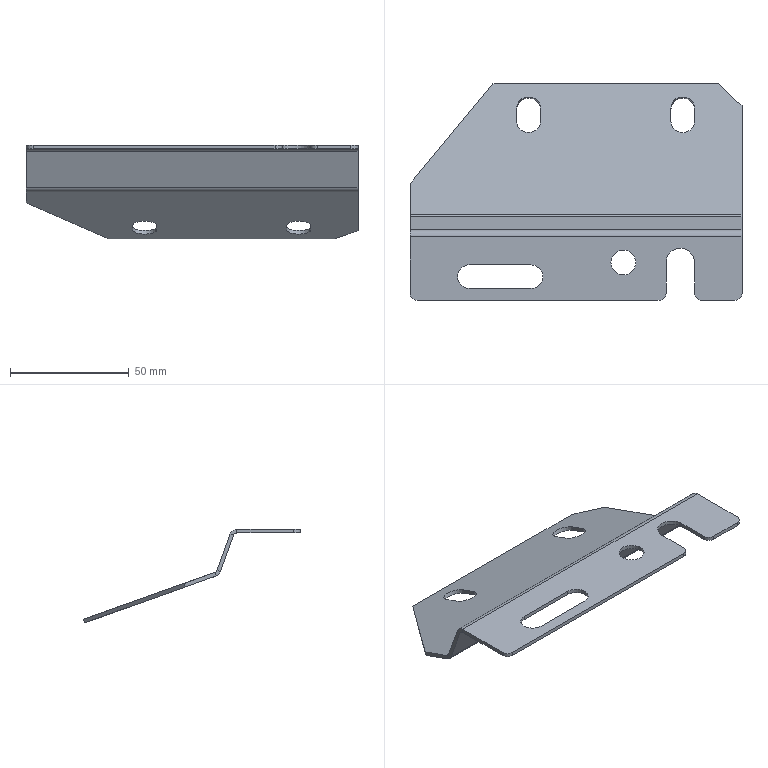Part | SolidWorks | features ICE 2, Fillet 1, FlatPattern 1, SMBaseFlange 1, SheetMetal 1 | 1 solid | 49 faces | box 140 x 91.5 x 39.507 mm | volume 21022 mm3 | plane 29 | cylinder 20 | commonest cylinder face diameters 10 x9 6 x4 3 x2 6.2 x2 10.5 x2 12 x1
STEP:
#1=CARTESIAN_POINT('',(95.25,16.,0.));
#2=VERTEX_POINT('',#1);
#3=CARTESIAN_POINT('',(84.75,16.,0.));
#4=VERTEX_POINT('',#3);
#5=CARTESIAN_POINT('',(90.,16.,0.));
#6=DIRECTION('',(0.,0.,-1.));
#7=DIRECTION('',(1.,0.,0.));
#8=AXIS2_PLACEMENT_3D('',#5,#6,#7);
#9=CIRCLE('',#8,5.25);
#10=EDGE_CURVE('',#2,#4,#9,.T.);
#11=ORIENTED_EDGE('',*,*,#10,.F.);
#12=CARTESIAN_POINT('',(95.25,16.,-1.6));
#13=VERTEX_POINT('',#12);
#14=CARTESIAN_POINT('',(95.25,16.,0.001));
#15=DIRECTION('',(0.,0.,-1.));
#16=VECTOR('',#15,1000.);
#17=LINE('',#14,#16);
#18=EDGE_CURVE('',#2,#13,#17,.T.);
#19=ORIENTED_EDGE('',*,*,#18,.T.);
#20=CARTESIAN_POINT('',(84.75,16.,-1.6));
#21=VERTEX_POINT('',#20);
#22=CARTESIAN_POINT('',(90.,16.,-1.6));
#23=DIRECTION('',(0.,0.,-1.));
#24=DIRECTION('',(-1.,0.,0.));
#25=AXIS2_PLACEMENT_3D('',#22,#23,#24);
#26=CIRCLE('',#25,5.25);
#27=EDGE_CURVE('',#13,#21,#26,.T.);
#28=ORIENTED_EDGE('',*,*,#27,.T.);
#29=CARTESIAN_POINT('',(84.75,16.,0.001));
#30=DIRECTION('',(0.,0.,-1.));
#31=VECTOR('',#30,1000.);
#32=LINE('',#29,#31);
#33=EDGE_CURVE('',#4,#21,#32,.T.);
#34=ORIENTED_EDGE('',*,*,#33,.F.);
#35=EDGE_LOOP('',(#11,#19,#28,#34));
#36=FACE_OUTER_BOUND('',#35,.T.);
#37=CARTESIAN_POINT('',(90.,16.,0.001));
#38=DIRECTION('',(0.,0.,-1.));
#39=DIRECTION('',(-1.,0.,0.));
#40=AXIS2_PLACEMENT_3D('',#37,#38,#39);
#41=CYLINDRICAL_SURFACE('',#40,5.25);
#42=ADVANCED_FACE('',(#36),#41,.F.);
#43=CARTESIAN_POINT('',(20.,10.,0.));
#44=VERTEX_POINT('',#43);
#45=CARTESIAN_POINT('',(25.,15.,0.));
#46=VERTEX_POINT('',#45);
#47=CARTESIAN_POINT('',(25.,10.,0.));
#48=DIRECTION('',(0.,0.,-1.));
#49=DIRECTION('',(1.,0.,0.));
#50=AXIS2_PLACEMENT_3D('',#47,#48,#49);
#51=CIRCLE('',#50,5.);
#52=EDGE_CURVE('',#44,#46,#51,.T.);
#53=ORIENTED_EDGE('',*,*,#52,.F.);
#54=CARTESIAN_POINT('',(20.,10.,-1.6));
#55=VERTEX_POINT('',#54);
#56=CARTESIAN_POINT('',(20.,10.,0.001));
#57=DIRECTION('',(0.,0.,-1.));
#58=VECTOR('',#57,1000.);
#59=LINE('',#56,#58);
#60=EDGE_CURVE('',#44,#55,#59,.T.);
#61=ORIENTED_EDGE('',*,*,#60,.T.);
#62=CARTESIAN_POINT('',(25.,15.,-1.6));
#63=VERTEX_POINT('',#62);
#64=CARTESIAN_POINT('',(25.,10.,-1.6));
#65=DIRECTION('',(0.,0.,-1.));
#66=DIRECTION('',(-1.,0.,0.));
#67=AXIS2_PLACEMENT_3D('',#64,#65,#66);
#68=CIRCLE('',#67,5.);
#69=EDGE_CURVE('',#55,#63,#68,.T.);
#70=ORIENTED_EDGE('',*,*,#69,.T.);
#71=CARTESIAN_POINT('',(25.,15.,0.001));
#72=DIRECTION('',(0.,0.,-1.));
#73=VECTOR('',#72,1000.);
#74=LINE('',#71,#73);
#75=EDGE_CURVE('',#46,#63,#74,.T.);
#76=ORIENTED_EDGE('',*,*,#75,.F.);
#77=EDGE_LOOP('',(#53,#61,#70,#76));
#78=FACE_OUTER_BOUND('',#77,.T.);
#79=CARTESIAN_POINT('',(25.,10.,0.001));
#80=DIRECTION('',(0.,0.,-1.));
#81=DIRECTION('',(-1.,0.,0.));
#82=AXIS2_PLACEMENT_3D('',#79,#80,#81);
#83=CYLINDRICAL_SURFACE('',#82,5.);
#84=ADVANCED_FACE('',(#78),#83,.F.);
#85=CARTESIAN_POINT('',(55.,74.952,-33.789));
#86=VERTEX_POINT('',#85);
#87=CARTESIAN_POINT('',(50.,70.244,-32.107));
#88=VERTEX_POINT('',#87);
#89=CARTESIAN_POINT('',(50.,74.952,-33.789));
#90=DIRECTION('',(0.,-0.3363,-0.9417));
#91=DIRECTION('',(0.,-0.9417,0.3363));
#92=AXIS2_PLACEMENT_3D('',#89,#90,#91);
#93=CIRCLE('',#92,5.);
#94=EDGE_CURVE('',#86,#88,#93,.T.);
#95=ORIENTED_EDGE('',*,*,#94,.T.);
#96=CARTESIAN_POINT('',(50.,70.782,-30.601));
#97=VERTEX_POINT('',#96);
#98=CARTESIAN_POINT('',(50.,70.244,-32.107));
#99=DIRECTION('',(0.,0.3363,0.9417));
#100=VECTOR('',#99,1000.);
#101=LINE('',#98,#100);
#102=EDGE_CURVE('',#88,#97,#101,.T.);
#103=ORIENTED_EDGE('',*,*,#102,.T.);
#104=CARTESIAN_POINT('',(55.,75.49,-32.282));
#105=VERTEX_POINT('',#104);
#106=CARTESIAN_POINT('',(50.,75.49,-32.282));
#107=DIRECTION('',(0.,-0.3363,-0.9417));
#108=DIRECTION('',(0.,-0.9417,0.3363));
#109=AXIS2_PLACEMENT_3D('',#106,#107,#108);
#110=CIRCLE('',#109,5.);
#111=EDGE_CURVE('',#105,#97,#110,.T.);
#112=ORIENTED_EDGE('',*,*,#111,.F.);
#113=CARTESIAN_POINT('',(55.,74.952,-33.789));
#114=DIRECTION('',(0.,0.3363,0.9417));
#115=VECTOR('',#114,1000.);
#116=LINE('',#113,#115);
#117=EDGE_CURVE('',#86,#105,#116,.T.);
#118=ORIENTED_EDGE('',*,*,#117,.F.);
#119=EDGE_LOOP('',(#95,#103,#112,#118));
#120=FACE_OUTER_BOUND('',#119,.T.);
#121=CARTESIAN_POINT('',(50.,74.952,-33.789));
#122=DIRECTION('',(0.,0.3363,0.9417));
#123=DIRECTION('',(0.,-0.9417,0.3363));
#124=AXIS2_PLACEMENT_3D('',#121,#122,#123);
#125=CYLINDRICAL_SURFACE('',#124,5.);
#126=ADVANCED_FACE('',(#120),#125,.F.);
#127=CARTESIAN_POINT('',(120.,74.952,-33.789));
#128=VERTEX_POINT('',#127);
#129=CARTESIAN_POINT('',(115.,70.244,-32.107));
#130=VERTEX_POINT('',#129);
#131=CARTESIAN_POINT('',(115.,74.952,-33.789));
#132=DIRECTION('',(0.,-0.3363,-0.9417));
#133=DIRECTION('',(0.,-0.9417,0.3363));
#134=AXIS2_PLACEMENT_3D('',#131,#132,#133);
#135=CIRCLE('',#134,5.);
#136=EDGE_CURVE('',#128,#130,#135,.T.);
#137=ORIENTED_EDGE('',*,*,#136,.T.);
#138=CARTESIAN_POINT('',(115.,70.782,-30.601));
#139=VERTEX_POINT('',#138);
#140=CARTESIAN_POINT('',(115.,70.244,-32.107));
#141=DIRECTION('',(0.,0.3363,0.9417));
#142=VECTOR('',#141,1000.);
#143=LINE('',#140,#142);
#144=EDGE_CURVE('',#130,#139,#143,.T.);
#145=ORIENTED_EDGE('',*,*,#144,.T.);
#146=CARTESIAN_POINT('',(120.,75.49,-32.282));
#147=VERTEX_POINT('',#146);
#148=CARTESIAN_POINT('',(115.,75.49,-32.282));
#149=DIRECTION('',(0.,-0.3363,-0.9417));
#150=DIRECTION('',(0.,-0.9417,0.3363));
#151=AXIS2_PLACEMENT_3D('',#148,#149,#150);
#152=CIRCLE('',#151,5.);
#153=EDGE_CURVE('',#147,#139,#152,.T.);
#154=ORIENTED_EDGE('',*,*,#153,.F.);
#155=CARTESIAN_POINT('',(120.,74.952,-33.789));
#156=DIRECTION('',(0.,0.3363,0.9417));
#157=VECTOR('',#156,1000.);
#158=LINE('',#155,#157);
#159=EDGE_CURVE('',#128,#147,#158,.T.);
#160=ORIENTED_EDGE('',*,*,#159,.F.);
#161=EDGE_LOOP('',(#137,#145,#154,#160));
#162=FACE_OUTER_BOUND('',#161,.T.);
#163=CARTESIAN_POINT('',(115.,74.952,-33.789));
#164=DIRECTION('',(0.,0.3363,0.9417));
#165=DIRECTION('',(0.,-0.9417,0.3363));
#166=AXIS2_PLACEMENT_3D('',#163,#164,#165);
#167=CYLINDRICAL_SURFACE('',#166,5.);
#168=ADVANCED_FACE('',(#162),#167,.F.);
#169=CARTESIAN_POINT('',(137.,0.,0.));
#170=VERTEX_POINT('',#169);
#171=CARTESIAN_POINT('',(123.,0.,0.));
#172=VERTEX_POINT('',#171);
#173=CARTESIAN_POINT('',(140.,0.,0.));
#174=DIRECTION('',(-1.,0.,0.));
#175=VECTOR('',#174,1000.);
#176=LINE('',#173,#175);
#177=EDGE_CURVE('',#170,#172,#176,.T.);
#178=ORIENTED_EDGE('',*,*,#177,.T.);
#179=CARTESIAN_POINT('',(123.,0.,-1.6));
#180=VERTEX_POINT('',#179);
#181=CARTESIAN_POINT('',(123.,0.,-1.6));
#182=DIRECTION('',(0.,0.,-1.));
#183=VECTOR('',#182,1000.);
#184=LINE('',#181,#183);
#185=EDGE_CURVE('',#172,#180,#184,.T.);
#186=ORIENTED_EDGE('',*,*,#185,.T.);
#187=CARTESIAN_POINT('',(137.,0.,-1.6));
#188=VERTEX_POINT('',#187);
#189=CARTESIAN_POINT('',(140.,0.,-1.6));
#190=DIRECTION('',(-1.,0.,0.));
#191=VECTOR('',#190,1000.);
#192=LINE('',#189,#191);
#193=EDGE_CURVE('',#188,#180,#192,.T.);
#194=ORIENTED_EDGE('',*,*,#193,.F.);
#195=CARTESIAN_POINT('',(137.,0.,0.));
#196=DIRECTION('',(0.,0.,1.));
#197=VECTOR('',#196,1000.);
#198=LINE('',#195,#197);
#199=EDGE_CURVE('',#188,#170,#198,.T.);
#200=ORIENTED_EDGE('',*,*,#199,.T.);
#201=EDGE_LOOP('',(#178,#186,#194,#200));
#202=FACE_OUTER_BOUND('',#201,.T.);
#203=CARTESIAN_POINT('',(140.,0.,-1.6));
#204=DIRECTION('',(0.,-1.,0.));
#205=DIRECTION('',(0.,0.,-1.));
#206=AXIS2_PLACEMENT_3D('',#203,#204,#205);
#207=PLANE('',#206);
#208=ADVANCED_FACE('',(#202),#207,.T.);
#209=CARTESIAN_POINT('',(140.,35.628,-19.745));
#210=VERTEX_POINT('',#209);
#211=CARTESIAN_POINT('',(140.,81.544,-36.143));
#212=VERTEX_POINT('',#211);
#213=CARTESIAN_POINT('',(140.,34.962,-19.507));
#214=DIRECTION('',(0.,0.9417,-0.3363));
#215=VECTOR('',#214,1000.);
#216=LINE('',#213,#215);
#217=EDGE_CURVE('',#210,#212,#216,.T.);
#218=ORIENTED_EDGE('',*,*,#217,.T.);
#219=CARTESIAN_POINT('',(140.,82.083,-34.637));
#220=VERTEX_POINT('',#219);
#221=CARTESIAN_POINT('',(140.,81.544,-36.143));
#222=DIRECTION('',(0.,0.3363,0.9417));
#223=VECTOR('',#222,1000.);
#224=LINE('',#221,#223);
#225=EDGE_CURVE('',#212,#220,#224,.T.);
#226=ORIENTED_EDGE('',*,*,#225,.T.);
#227=CARTESIAN_POINT('',(140.,36.166,-18.238));
#228=VERTEX_POINT('',#227);
#229=CARTESIAN_POINT('',(140.,35.5,-18.));
#230=DIRECTION('',(0.,0.9417,-0.3363));
#231=VECTOR('',#230,1000.);
#232=LINE('',#229,#231);
#233=EDGE_CURVE('',#228,#220,#232,.T.);
#234=ORIENTED_EDGE('',*,*,#233,.F.);
#235=CARTESIAN_POINT('',(140.,36.166,-18.238));
#236=DIRECTION('',(0.,-0.3363,-0.9417));
#237=VECTOR('',#236,1000.);
#238=LINE('',#235,#237);
#239=EDGE_CURVE('',#228,#210,#238,.T.);
#240=ORIENTED_EDGE('',*,*,#239,.T.);
#241=EDGE_LOOP('',(#218,#226,#234,#240));
#242=FACE_OUTER_BOUND('',#241,.T.);
#243=CARTESIAN_POINT('',(140.,33.755,-17.878));
#244=DIRECTION('',(1.,0.,0.));
#245=DIRECTION('',(0.,0.,-1.));
#246=AXIS2_PLACEMENT_3D('',#243,#244,#245);
#247=PLANE('',#246);
#248=ADVANCED_FACE('',(#242),#247,.T.);
#249=ORIENTED_EDGE('',*,*,#94,.F.);
#250=CARTESIAN_POINT('',(55.,80.603,-35.807));
#251=VERTEX_POINT('',#250);
#252=CARTESIAN_POINT('',(55.,80.603,-35.807));
#253=DIRECTION('',(0.,-0.9417,0.3363));
#254=VECTOR('',#253,1000.);
#255=LINE('',#252,#254);
#256=EDGE_CURVE('',#251,#86,#255,.T.);
#257=ORIENTED_EDGE('',*,*,#256,.F.);
#258=CARTESIAN_POINT('',(45.,80.603,-35.807));
#259=VERTEX_POINT('',#258);
#260=CARTESIAN_POINT('',(50.,80.603,-35.807));
#261=DIRECTION('',(0.,-0.3363,-0.9417));
#262=DIRECTION('',(0.,-0.9417,0.3363));
#263=AXIS2_PLACEMENT_3D('',#260,#261,#262);
#264=CIRCLE('',#263,5.);
#265=EDGE_CURVE('',#259,#251,#264,.T.);
#266=ORIENTED_EDGE('',*,*,#265,.F.);
#267=CARTESIAN_POINT('',(45.,74.952,-33.789));
#268=VERTEX_POINT('',#267);
#269=CARTESIAN_POINT('',(45.,80.603,-35.807));
#270=DIRECTION('',(0.,0.9417,-0.3363));
#271=VECTOR('',#270,1000.);
#272=LINE('',#269,#271);
#273=EDGE_CURVE('',#268,#259,#272,.T.);
#274=ORIENTED_EDGE('',*,*,#273,.F.);
#275=CARTESIAN_POINT('',(50.,74.952,-33.789));
#276=DIRECTION('',(0.,-0.3363,-0.9417));
#277=DIRECTION('',(0.,-0.9417,0.3363));
#278=AXIS2_PLACEMENT_3D('',#275,#276,#277);
#279=CIRCLE('',#278,5.);
#280=EDGE_CURVE('',#88,#268,#279,.T.);
#281=ORIENTED_EDGE('',*,*,#280,.F.);
#282=EDGE_LOOP('',(#249,#257,#266,#274,#281));
#283=FACE_BOUND('',#282,.T.);
#284=ORIENTED_EDGE('',*,*,#136,.F.);
#285=CARTESIAN_POINT('',(120.,80.603,-35.807));
#286=VERTEX_POINT('',#285);
#287=CARTESIAN_POINT('',(120.,80.603,-35.807));
#288=DIRECTION('',(0.,-0.9417,0.3363));
#289=VECTOR('',#288,1000.);
#290=LINE('',#287,#289);
#291=EDGE_CURVE('',#286,#128,#290,.T.);
#292=ORIENTED_EDGE('',*,*,#291,.F.);
#293=CARTESIAN_POINT('',(110.,80.603,-35.807));
#294=VERTEX_POINT('',#293);
#295=CARTESIAN_POINT('',(115.,80.603,-35.807));
#296=DIRECTION('',(0.,-0.3363,-0.9417));
#297=DIRECTION('',(0.,-0.9417,0.3363));
#298=AXIS2_PLACEMENT_3D('',#295,#296,#297);
#299=CIRCLE('',#298,5.);
#300=EDGE_CURVE('',#294,#286,#299,.T.);
#301=ORIENTED_EDGE('',*,*,#300,.F.);
#302=CARTESIAN_POINT('',(110.,74.952,-33.789));
#303=VERTEX_POINT('',#302);
#304=CARTESIAN_POINT('',(110.,80.603,-35.807));
#305=DIRECTION('',(0.,0.9417,-0.3363));
#306=VECTOR('',#305,1000.);
#307=LINE('',#304,#306);
#308=EDGE_CURVE('',#303,#294,#307,.T.);
#309=ORIENTED_EDGE('',*,*,#308,.F.);
#310=CARTESIAN_POINT('',(115.,74.952,-33.789));
#311=DIRECTION('',(0.,-0.3363,-0.9417));
#312=DIRECTION('',(0.,-0.9417,0.3363));
#313=AXIS2_PLACEMENT_3D('',#310,#311,#312);
#314=CIRCLE('',#313,5.);
#315=EDGE_CURVE('',#130,#303,#314,.T.);
#316=ORIENTED_EDGE('',*,*,#315,.F.);
#317=EDGE_LOOP('',(#284,#292,#301,#309,#316));
#318=FACE_BOUND('',#317,.T.);
#319=CARTESIAN_POINT('',(130.,90.962,-39.507));
#320=VERTEX_POINT('',#319);
#321=CARTESIAN_POINT('',(130.,90.962,-39.507));
#322=DIRECTION('',(-0.7071,0.6659,-0.2378));
#323=VECTOR('',#322,1000.);
#324=LINE('',#321,#323);
#325=EDGE_CURVE('',#212,#320,#324,.T.);
#326=ORIENTED_EDGE('',*,*,#325,.F.);
#327=ORIENTED_EDGE('',*,*,#217,.F.);
#328=CARTESIAN_POINT('',(0.,35.628,-19.745));
#329=VERTEX_POINT('',#328);
#330=CARTESIAN_POINT('',(140.,35.628,-19.745));
#331=DIRECTION('',(-1.,0.,0.));
#332=VECTOR('',#331,1000.);
#333=LINE('',#330,#332);
#334=EDGE_CURVE('',#210,#329,#333,.T.);
#335=ORIENTED_EDGE('',*,*,#334,.T.);
#336=CARTESIAN_POINT('',(0.,48.583,-24.372));
#337=VERTEX_POINT('',#336);
#338=CARTESIAN_POINT('',(0.,34.962,-19.507));
#339=DIRECTION('',(0.,0.9417,-0.3363));
#340=VECTOR('',#339,1000.);
#341=LINE('',#338,#340);
#342=EDGE_CURVE('',#329,#337,#341,.T.);
#343=ORIENTED_EDGE('',*,*,#342,.T.);
#344=CARTESIAN_POINT('',(35.,90.962,-39.507));
#345=VERTEX_POINT('',#344);
#346=CARTESIAN_POINT('',(35.,90.962,-39.507));
#347=DIRECTION('',(-0.6139,-0.7434,0.2655));
#348=VECTOR('',#347,1000.);
#349=LINE('',#346,#348);
#350=EDGE_CURVE('',#345,#337,#349,.T.);
#351=ORIENTED_EDGE('',*,*,#350,.F.);
#352=CARTESIAN_POINT('',(140.,90.962,-39.507));
#353=DIRECTION('',(-1.,0.,0.));
#354=VECTOR('',#353,1000.);
#355=LINE('',#352,#354);
#356=EDGE_CURVE('',#320,#345,#355,.T.);
#357=ORIENTED_EDGE('',*,*,#356,.F.);
#358=EDGE_LOOP('',(#326,#327,#335,#343,#351,#357));
#359=FACE_OUTER_BOUND('',#358,.T.);
#360=CARTESIAN_POINT('',(140.,34.962,-19.507));
#361=DIRECTION('',(0.,0.3363,0.9417));
#362=DIRECTION('',(0.,-0.9417,0.3363));
#363=AXIS2_PLACEMENT_3D('',#360,#361,#362);
#364=PLANE('',#363);
#365=ADVANCED_FACE('',(#283,#318,#359),#364,.F.);
#366=CARTESIAN_POINT('',(130.,91.5,-38.));
#367=VERTEX_POINT('',#366);
#368=CARTESIAN_POINT('',(35.,91.5,-38.));
#369=VERTEX_POINT('',#368);
#370=CARTESIAN_POINT('',(140.,91.5,-38.));
#371=DIRECTION('',(-1.,0.,0.));
#372=VECTOR('',#371,1000.);
#373=LINE('',#370,#372);
#374=EDGE_CURVE('',#367,#369,#373,.T.);
#375=ORIENTED_EDGE('',*,*,#374,.F.);
#376=CARTESIAN_POINT('',(130.,90.962,-39.507));
#377=DIRECTION('',(0.,0.3363,0.9417));
#378=VECTOR('',#377,1000.);
#379=LINE('',#376,#378);
#380=EDGE_CURVE('',#320,#367,#379,.T.);
#381=ORIENTED_EDGE('',*,*,#380,.F.);
#382=ORIENTED_EDGE('',*,*,#356,.T.);
#383=CARTESIAN_POINT('',(35.,90.962,-39.507));
#384=DIRECTION('',(0.,0.3363,0.9417));
#385=VECTOR('',#384,1000.);
#386=LINE('',#383,#385);
#387=EDGE_CURVE('',#345,#369,#386,.T.);
#388=ORIENTED_EDGE('',*,*,#387,.T.);
#389=EDGE_LOOP('',(#375,#381,#382,#388));
#390=FACE_OUTER_BOUND('',#389,.T.);
#391=CARTESIAN_POINT('',(140.,91.5,-38.));
#392=DIRECTION('',(0.,0.9417,-0.3363));
#393=DIRECTION('',(0.,0.3363,0.9417));
#394=AXIS2_PLACEMENT_3D('',#391,#392,#393);
#395=PLANE('',#394);
#396=ADVANCED_FACE('',(#390),#395,.T.);
#397=CARTESIAN_POINT('',(120.,81.141,-34.3));
#398=VERTEX_POINT('',#397);
#399=CARTESIAN_POINT('',(120.,35.5,-18.));
#400=DIRECTION('',(0.,-0.9417,0.3363));
#401=VECTOR('',#400,1000.);
#402=LINE('',#399,#401);
#403=EDGE_CURVE('',#398,#147,#402,.T.);
#404=ORIENTED_EDGE('',*,*,#403,.T.);
#405=ORIENTED_EDGE('',*,*,#153,.T.);
#406=CARTESIAN_POINT('',(110.,75.49,-32.282));
#407=VERTEX_POINT('',#406);
#408=CARTESIAN_POINT('',(115.,75.49,-32.282));
#409=DIRECTION('',(0.,-0.3363,-0.9417));
#410=DIRECTION('',(0.,-0.9417,0.3363));
#411=AXIS2_PLACEMENT_3D('',#408,#409,#410);
#412=CIRCLE('',#411,5.);
#413=EDGE_CURVE('',#139,#407,#412,.T.);
#414=ORIENTED_EDGE('',*,*,#413,.T.);
#415=CARTESIAN_POINT('',(110.,81.141,-34.3));
#416=VERTEX_POINT('',#415);
#417=CARTESIAN_POINT('',(110.,35.5,-18.));
#418=DIRECTION('',(0.,0.9417,-0.3363));
#419=VECTOR('',#418,1000.);
#420=LINE('',#417,#419);
#421=EDGE_CURVE('',#407,#416,#420,.T.);
#422=ORIENTED_EDGE('',*,*,#421,.T.);
#423=CARTESIAN_POINT('',(115.,81.141,-34.3));
#424=DIRECTION('',(0.,-0.3363,-0.9417));
#425=DIRECTION('',(0.,-0.9417,0.3363));
#426=AXIS2_PLACEMENT_3D('',#423,#424,#425);
#427=CIRCLE('',#426,5.);
#428=EDGE_CURVE('',#416,#398,#427,.T.);
#429=ORIENTED_EDGE('',*,*,#428,.T.);
#430=EDGE_LOOP('',(#404,#405,#414,#422,#429));
#431=FACE_BOUND('',#430,.T.);
#432=CARTESIAN_POINT('',(55.,81.141,-34.3));
#433=VERTEX_POINT('',#432);
#434=CARTESIAN_POINT('',(55.,35.5,-18.));
#435=DIRECTION('',(0.,-0.9417,0.3363));
#436=VECTOR('',#435,1000.);
#437=LINE('',#434,#436);
#438=EDGE_CURVE('',#433,#105,#437,.T.);
#439=ORIENTED_EDGE('',*,*,#438,.T.);
#440=ORIENTED_EDGE('',*,*,#111,.T.);
#441=CARTESIAN_POINT('',(45.,75.49,-32.282));
#442=VERTEX_POINT('',#441);
#443=CARTESIAN_POINT('',(50.,75.49,-32.282));
#444=DIRECTION('',(0.,-0.3363,-0.9417));
#445=DIRECTION('',(0.,-0.9417,0.3363));
#446=AXIS2_PLACEMENT_3D('',#443,#444,#445);
#447=CIRCLE('',#446,5.);
#448=EDGE_CURVE('',#97,#442,#447,.T.);
#449=ORIENTED_EDGE('',*,*,#448,.T.);
#450=CARTESIAN_POINT('',(45.,81.141,-34.3));
#451=VERTEX_POINT('',#450);
#452=CARTESIAN_POINT('',(45.,35.5,-18.));
#453=DIRECTION('',(0.,0.9417,-0.3363));
#454=VECTOR('',#453,1000.);
#455=LINE('',#452,#454);
#456=EDGE_CURVE('',#442,#451,#455,.T.);
#457=ORIENTED_EDGE('',*,*,#456,.T.);
#458=CARTESIAN_POINT('',(50.,81.141,-34.3));
#459=DIRECTION('',(0.,-0.3363,-0.9417));
#460=DIRECTION('',(0.,-0.9417,0.3363));
#461=AXIS2_PLACEMENT_3D('',#458,#459,#460);
#462=CIRCLE('',#461,5.);
#463=EDGE_CURVE('',#451,#433,#462,.T.);
#464=ORIENTED_EDGE('',*,*,#463,.T.);
#465=EDGE_LOOP('',(#439,#440,#449,#457,#464));
#466=FACE_BOUND('',#465,.T.);
#467=ORIENTED_EDGE('',*,*,#233,.T.);
#468=CARTESIAN_POINT('',(130.,91.5,-38.));
#469=DIRECTION('',(-0.7071,0.6659,-0.2378));
#470=VECTOR('',#469,1000.);
#471=LINE('',#468,#470);
#472=EDGE_CURVE('',#220,#367,#471,.T.);
#473=ORIENTED_EDGE('',*,*,#472,.T.);
#474=ORIENTED_EDGE('',*,*,#374,.T.);
#475=CARTESIAN_POINT('',(0.,49.122,-22.865));
#476=VERTEX_POINT('',#475);
#477=CARTESIAN_POINT('',(35.,91.5,-38.));
#478=DIRECTION('',(-0.6139,-0.7434,0.2655));
#479=VECTOR('',#478,1000.);
#480=LINE('',#477,#479);
#481=EDGE_CURVE('',#369,#476,#480,.T.);
#482=ORIENTED_EDGE('',*,*,#481,.T.);
#483=CARTESIAN_POINT('',(0.,36.166,-18.238));
#484=VERTEX_POINT('',#483);
#485=CARTESIAN_POINT('',(0.,35.5,-18.));
#486=DIRECTION('',(0.,0.9417,-0.3363));
#487=VECTOR('',#486,1000.);
#488=LINE('',#485,#487);
#489=EDGE_CURVE('',#484,#476,#488,.T.);
#490=ORIENTED_EDGE('',*,*,#489,.F.);
#491=CARTESIAN_POINT('',(140.,36.166,-18.238));
#492=DIRECTION('',(-1.,0.,0.));
#493=VECTOR('',#492,1000.);
#494=LINE('',#491,#493);
#495=EDGE_CURVE('',#228,#484,#494,.T.);
#496=ORIENTED_EDGE('',*,*,#495,.F.);
#497=EDGE_LOOP('',(#467,#473,#474,#482,#490,#496));
#498=FACE_OUTER_BOUND('',#497,.T.);
#499=CARTESIAN_POINT('',(140.,35.5,-18.));
#500=DIRECTION('',(0.,0.3363,0.9417));
#501=DIRECTION('',(0.,-0.9417,0.3363));
#502=AXIS2_PLACEMENT_3D('',#499,#500,#501);
#503=PLANE('',#502);
#504=ADVANCED_FACE('',(#431,#466,#498),#503,.T.);
#505=ORIENTED_EDGE('',*,*,#489,.T.);
#506=CARTESIAN_POINT('',(0.,48.583,-24.372));
#507=DIRECTION('',(0.,0.3363,0.9417));
#508=VECTOR('',#507,1000.);
#509=LINE('',#506,#508);
#510=EDGE_CURVE('',#337,#476,#509,.T.);
#511=ORIENTED_EDGE('',*,*,#510,.F.);
#512=ORIENTED_EDGE('',*,*,#342,.F.);
#513=CARTESIAN_POINT('',(0.,35.628,-19.745));
#514=DIRECTION('',(0.,0.3363,0.9417));
#515=VECTOR('',#514,1000.);
#516=LINE('',#513,#515);
#517=EDGE_CURVE('',#329,#484,#516,.T.);
#518=ORIENTED_EDGE('',*,*,#517,.T.);
#519=EDGE_LOOP('',(#505,#511,#512,#518));
#520=FACE_OUTER_BOUND('',#519,.T.);
#521=CARTESIAN_POINT('',(0.,36.671,-16.825));
#522=DIRECTION('',(-1.,0.,0.));
#523=DIRECTION('',(0.,0.,1.));
#524=AXIS2_PLACEMENT_3D('',#521,#522,#523);
#525=PLANE('',#524);
#526=ADVANCED_FACE('',(#520),#525,.T.);
#527=CARTESIAN_POINT('',(140.,29.739,-2.047));
#528=VERTEX_POINT('',#527);
#529=CARTESIAN_POINT('',(140.,28.234,-2.591));
#530=VERTEX_POINT('',#529);
#531=CARTESIAN_POINT('',(140.,29.739,-2.047));
#532=DIRECTION('',(0.,-0.9406,-0.3396));
#533=VECTOR('',#532,1000.);
#534=LINE('',#531,#533);
#535=EDGE_CURVE('',#528,#530,#534,.T.);
#536=ORIENTED_EDGE('',*,*,#535,.F.);
#537=CARTESIAN_POINT('',(140.,26.824,0.));
#538=VERTEX_POINT('',#537);
#539=CARTESIAN_POINT('',(140.,26.824,-3.1));
#540=DIRECTION('',(-1.,0.,0.));
#541=DIRECTION('',(0.,0.,-1.));
#542=AXIS2_PLACEMENT_3D('',#539,#540,#541);
#543=CIRCLE('',#542,3.1);
#544=EDGE_CURVE('',#538,#528,#543,.T.);
#545=ORIENTED_EDGE('',*,*,#544,.F.);
#546=CARTESIAN_POINT('',(140.,26.824,-1.6));
#547=VERTEX_POINT('',#546);
#548=CARTESIAN_POINT('',(140.,26.824,-1.6));
#549=DIRECTION('',(0.,0.,1.));
#550=VECTOR('',#549,1000.);
#551=LINE('',#548,#550);
#552=EDGE_CURVE('',#547,#538,#551,.T.);
#553=ORIENTED_EDGE('',*,*,#552,.F.);
#554=CARTESIAN_POINT('',(140.,26.824,-3.1));
#555=DIRECTION('',(-1.,0.,0.));
#556=DIRECTION('',(0.,0.,-1.));
#557=AXIS2_PLACEMENT_3D('',#554,#555,#556);
#558=CIRCLE('',#557,1.5);
#559=EDGE_CURVE('',#547,#530,#558,.T.);
#560=ORIENTED_EDGE('',*,*,#559,.T.);
#561=EDGE_LOOP('',(#536,#545,#553,#560));
#562=FACE_OUTER_BOUND('',#561,.T.);
#563=CARTESIAN_POINT('',(140.,29.739,-2.047));
#564=DIRECTION('',(1.,0.,0.));
#565=DIRECTION('',(0.,0.,-1.));
#566=AXIS2_PLACEMENT_3D('',#563,#564,#565);
#567=PLANE('',#566);
#568=ADVANCED_FACE('',(#562),#567,.T.);
#569=CARTESIAN_POINT('',(140.,35.26,-17.335));
#570=VERTEX_POINT('',#569);
#571=CARTESIAN_POINT('',(140.,29.,0.));
#572=DIRECTION('',(0.,0.3396,-0.9406));
#573=VECTOR('',#572,1000.);
#574=LINE('',#571,#573);
#575=EDGE_CURVE('',#528,#570,#574,.T.);
#576=ORIENTED_EDGE('',*,*,#575,.F.);
#577=ORIENTED_EDGE('',*,*,#535,.T.);
#578=CARTESIAN_POINT('',(140.,33.755,-17.878));
#579=VERTEX_POINT('',#578);
#580=CARTESIAN_POINT('',(140.,27.495,-0.5434));
#581=DIRECTION('',(0.,0.3396,-0.9406));
#582=VECTOR('',#581,1000.);
#583=LINE('',#580,#582);
#584=EDGE_CURVE('',#530,#579,#583,.T.);
#585=ORIENTED_EDGE('',*,*,#584,.T.);
#586=CARTESIAN_POINT('',(140.,33.755,-17.878));
#587=DIRECTION('',(0.,0.9406,0.3396));
#588=VECTOR('',#587,1000.);
#589=LINE('',#586,#588);
#590=EDGE_CURVE('',#579,#570,#589,.T.);
#591=ORIENTED_EDGE('',*,*,#590,.T.);
#592=EDGE_LOOP('',(#576,#577,#585,#591));
#593=FACE_OUTER_BOUND('',#592,.T.);
#594=CARTESIAN_POINT('',(140.,26.824,-1.6));
#595=DIRECTION('',(1.,0.,0.));
#596=DIRECTION('',(0.,0.,-1.));
#597=AXIS2_PLACEMENT_3D('',#594,#595,#596);
#598=PLANE('',#597);
#599=ADVANCED_FACE('',(#593),#598,.T.);
#600=CARTESIAN_POINT('',(0.,26.824,0.));
#601=VERTEX_POINT('',#600);
#602=CARTESIAN_POINT('',(0.,26.824,-1.6));
#603=VERTEX_POINT('',#602);
#604=CARTESIAN_POINT('',(0.,26.824,0.));
#605=DIRECTION('',(0.,0.,-1.));
#606=VECTOR('',#605,1000.);
#607=LINE('',#604,#606);
#608=EDGE_CURVE('',#601,#603,#607,.T.);
#609=ORIENTED_EDGE('',*,*,#608,.F.);
#610=CARTESIAN_POINT('',(0.,29.739,-2.047));
#611=VERTEX_POINT('',#610);
#612=CARTESIAN_POINT('',(0.,26.824,-3.1));
#613=DIRECTION('',(-1.,0.,0.));
#614=DIRECTION('',(0.,0.,-1.));
#615=AXIS2_PLACEMENT_3D('',#612,#613,#614);
#616=CIRCLE('',#615,3.1);
#617=EDGE_CURVE('',#601,#611,#616,.T.);
#618=ORIENTED_EDGE('',*,*,#617,.T.);
#619=CARTESIAN_POINT('',(0.,28.234,-2.591));
#620=VERTEX_POINT('',#619);
#621=CARTESIAN_POINT('',(0.,28.234,-2.591));
#622=DIRECTION('',(0.,0.9406,0.3396));
#623=VECTOR('',#622,1000.);
#624=LINE('',#621,#623);
#625=EDGE_CURVE('',#620,#611,#624,.T.);
#626=ORIENTED_EDGE('',*,*,#625,.F.);
#627=CARTESIAN_POINT('',(0.,26.824,-3.1));
#628=DIRECTION('',(-1.,0.,0.));
#629=DIRECTION('',(0.,0.,-1.));
#630=AXIS2_PLACEMENT_3D('',#627,#628,#629);
#631=CIRCLE('',#630,1.5);
#632=EDGE_CURVE('',#603,#620,#631,.T.);
#633=ORIENTED_EDGE('',*,*,#632,.F.);
#634=EDGE_LOOP('',(#609,#618,#626,#633));
#635=FACE_OUTER_BOUND('',#634,.T.);
#636=CARTESIAN_POINT('',(0.,26.824,0.));
#637=DIRECTION('',(-1.,0.,0.));
#638=DIRECTION('',(0.,0.,1.));
#639=AXIS2_PLACEMENT_3D('',#636,#637,#638);
#640=PLANE('',#639);
#641=ADVANCED_FACE('',(#635),#640,.T.);
#642=CARTESIAN_POINT('',(0.,3.,-1.6));
#643=VERTEX_POINT('',#642);
#644=CARTESIAN_POINT('',(0.,0.,-1.6));
#645=DIRECTION('',(0.,1.,0.));
#646=VECTOR('',#645,1000.);
#647=LINE('',#644,#646);
#648=EDGE_CURVE('',#643,#603,#647,.T.);
#649=ORIENTED_EDGE('',*,*,#648,.F.);
#650=CARTESIAN_POINT('',(0.,3.,0.));
#651=VERTEX_POINT('',#650);
#652=CARTESIAN_POINT('',(0.,3.,-2.591));
#653=DIRECTION('',(0.,0.,1.));
#654=VECTOR('',#653,1000.);
#655=LINE('',#652,#654);
#656=EDGE_CURVE('',#643,#651,#655,.T.);
#657=ORIENTED_EDGE('',*,*,#656,.T.);
#658=CARTESIAN_POINT('',(0.,0.,0.));
#659=DIRECTION('',(0.,1.,0.));
#660=VECTOR('',#659,1000.);
#661=LINE('',#658,#660);
#662=EDGE_CURVE('',#651,#601,#661,.T.);
#663=ORIENTED_EDGE('',*,*,#662,.T.);
#664=ORIENTED_EDGE('',*,*,#608,.T.);
#665=EDGE_LOOP('',(#649,#657,#663,#664));
#666=FACE_OUTER_BOUND('',#665,.T.);
#667=CARTESIAN_POINT('',(0.,28.234,-2.591));
#668=DIRECTION('',(-1.,0.,0.));
#669=DIRECTION('',(0.,0.,1.));
#670=AXIS2_PLACEMENT_3D('',#667,#668,#669);
#671=PLANE('',#670);
#672=ADVANCED_FACE('',(#666),#671,.T.);
#673=ORIENTED_EDGE('',*,*,#239,.F.);
#674=CARTESIAN_POINT('',(140.,36.671,-16.825));
#675=DIRECTION('',(1.,0.,0.));
#676=DIRECTION('',(0.,0.,1.));
#677=AXIS2_PLACEMENT_3D('',#674,#675,#676);
#678=CIRCLE('',#677,1.5);
#679=EDGE_CURVE('',#570,#228,#678,.T.);
#680=ORIENTED_EDGE('',*,*,#679,.F.);
#681=ORIENTED_EDGE('',*,*,#590,.F.);
#682=CARTESIAN_POINT('',(140.,36.671,-16.825));
#683=DIRECTION('',(1.,0.,0.));
#684=DIRECTION('',(0.,0.,-1.));
#685=AXIS2_PLACEMENT_3D('',#682,#683,#684);
#686=CIRCLE('',#685,3.1);
#687=EDGE_CURVE('',#579,#210,#686,.T.);
#688=ORIENTED_EDGE('',*,*,#687,.T.);
#689=EDGE_LOOP('',(#673,#680,#681,#688));
#690=FACE_OUTER_BOUND('',#689,.T.);
#691=CARTESIAN_POINT('',(140.,36.166,-18.238));
#692=DIRECTION('',(1.,0.,0.));
#693=DIRECTION('',(0.,0.,-1.));
#694=AXIS2_PLACEMENT_3D('',#691,#692,#693);
#695=PLANE('',#694);
#696=ADVANCED_FACE('',(#690),#695,.T.);
#697=CARTESIAN_POINT('',(0.,35.26,-17.335));
#698=VERTEX_POINT('',#697);
#699=CARTESIAN_POINT('',(0.,33.755,-17.878));
#700=VERTEX_POINT('',#699);
#701=CARTESIAN_POINT('',(0.,35.26,-17.335));
#702=DIRECTION('',(0.,-0.9406,-0.3396));
#703=VECTOR('',#702,1000.);
#704=LINE('',#701,#703);
#705=EDGE_CURVE('',#698,#700,#704,.T.);
#706=ORIENTED_EDGE('',*,*,#705,.F.);
#707=CARTESIAN_POINT('',(0.,36.671,-16.825));
#708=DIRECTION('',(1.,0.,0.));
#709=DIRECTION('',(0.,0.,1.));
#710=AXIS2_PLACEMENT_3D('',#707,#708,#709);
#711=CIRCLE('',#710,1.5);
#712=EDGE_CURVE('',#698,#484,#711,.T.);
#713=ORIENTED_EDGE('',*,*,#712,.T.);
#714=ORIENTED_EDGE('',*,*,#517,.F.);
#715=CARTESIAN_POINT('',(0.,36.671,-16.825));
#716=DIRECTION('',(1.,0.,0.));
#717=DIRECTION('',(0.,0.,-1.));
#718=AXIS2_PLACEMENT_3D('',#715,#716,#717);
#719=CIRCLE('',#718,3.1);
#720=EDGE_CURVE('',#700,#329,#719,.T.);
#721=ORIENTED_EDGE('',*,*,#720,.F.);
#722=EDGE_LOOP('',(#706,#713,#714,#721));
#723=FACE_OUTER_BOUND('',#722,.T.);
#724=CARTESIAN_POINT('',(0.,35.26,-17.335));
#725=DIRECTION('',(-1.,0.,0.));
#726=DIRECTION('',(0.,0.,1.));
#727=AXIS2_PLACEMENT_3D('',#724,#725,#726);
#728=PLANE('',#727);
#729=ADVANCED_FACE('',(#723),#728,.T.);
#730=CARTESIAN_POINT('',(0.,29.,0.));
#731=DIRECTION('',(0.,0.3396,-0.9406));
#732=VECTOR('',#731,1000.);
#733=LINE('',#730,#732);
#734=EDGE_CURVE('',#611,#698,#733,.T.);
#735=ORIENTED_EDGE('',*,*,#734,.T.);
#736=ORIENTED_EDGE('',*,*,#705,.T.);
#737=CARTESIAN_POINT('',(0.,27.495,-0.5434));
#738=DIRECTION('',(0.,0.3396,-0.9406));
#739=VECTOR('',#738,1000.);
#740=LINE('',#737,#739);
#741=EDGE_CURVE('',#620,#700,#740,.T.);
#742=ORIENTED_EDGE('',*,*,#741,.F.);
#743=ORIENTED_EDGE('',*,*,#625,.T.);
#744=EDGE_LOOP('',(#735,#736,#742,#743));
#745=FACE_OUTER_BOUND('',#744,.T.);
#746=CARTESIAN_POINT('',(0.,35.628,-19.745));
#747=DIRECTION('',(-1.,0.,0.));
#748=DIRECTION('',(0.,0.,1.));
#749=AXIS2_PLACEMENT_3D('',#746,#747,#748);
#750=PLANE('',#749);
#751=ADVANCED_FACE('',(#745),#750,.T.);
#752=ORIENTED_EDGE('',*,*,#712,.F.);
#753=CARTESIAN_POINT('',(140.,35.26,-17.335));
#754=DIRECTION('',(-1.,0.,0.));
#755=VECTOR('',#754,1000.);
#756=LINE('',#753,#755);
#757=EDGE_CURVE('',#570,#698,#756,.T.);
#758=ORIENTED_EDGE('',*,*,#757,.F.);
#759=ORIENTED_EDGE('',*,*,#679,.T.);
#760=ORIENTED_EDGE('',*,*,#495,.T.);
#761=EDGE_LOOP('',(#752,#758,#759,#760));
#762=FACE_OUTER_BOUND('',#761,.T.);
#763=CARTESIAN_POINT('',(140.,36.671,-16.825));
#764=DIRECTION('',(-1.,0.,0.));
#765=DIRECTION('',(0.,0.,1.));
#766=AXIS2_PLACEMENT_3D('',#763,#764,#765);
#767=CYLINDRICAL_SURFACE('',#766,1.5);
#768=ADVANCED_FACE('',(#762),#767,.F.);
#769=ORIENTED_EDGE('',*,*,#734,.F.);
#770=CARTESIAN_POINT('',(140.,29.739,-2.047));
#771=DIRECTION('',(-1.,0.,0.));
#772=VECTOR('',#771,1000.);
#773=LINE('',#770,#772);
#774=EDGE_CURVE('',#528,#611,#773,.T.);
#775=ORIENTED_EDGE('',*,*,#774,.F.);
#776=ORIENTED_EDGE('',*,*,#575,.T.);
#777=ORIENTED_EDGE('',*,*,#757,.T.);
#778=EDGE_LOOP('',(#769,#775,#776,#777));
#779=FACE_OUTER_BOUND('',#778,.T.);
#780=CARTESIAN_POINT('',(140.,29.,0.));
#781=DIRECTION('',(0.,0.9406,0.3396));
#782=DIRECTION('',(0.,-0.3396,0.9406));
#783=AXIS2_PLACEMENT_3D('',#780,#781,#782);
#784=PLANE('',#783);
#785=ADVANCED_FACE('',(#779),#784,.T.);
#786=ORIENTED_EDGE('',*,*,#617,.F.);
#787=CARTESIAN_POINT('',(140.,26.824,0.));
#788=DIRECTION('',(-1.,0.,0.));
#789=VECTOR('',#788,1000.);
#790=LINE('',#787,#789);
#791=EDGE_CURVE('',#538,#601,#790,.T.);
#792=ORIENTED_EDGE('',*,*,#791,.F.);
#793=ORIENTED_EDGE('',*,*,#544,.T.);
#794=ORIENTED_EDGE('',*,*,#774,.T.);
#795=EDGE_LOOP('',(#786,#792,#793,#794));
#796=FACE_OUTER_BOUND('',#795,.T.);
#797=CARTESIAN_POINT('',(140.,26.824,-3.1));
#798=DIRECTION('',(-1.,0.,0.));
#799=DIRECTION('',(0.,0.,1.));
#800=AXIS2_PLACEMENT_3D('',#797,#798,#799);
#801=CYLINDRICAL_SURFACE('',#800,3.1);
#802=ADVANCED_FACE('',(#796),#801,.T.);
#803=ORIENTED_EDGE('',*,*,#662,.F.);
#804=CARTESIAN_POINT('',(3.,0.,0.));
#805=VERTEX_POINT('',#804);
#806=CARTESIAN_POINT('',(3.,3.,0.));
#807=DIRECTION('',(0.,0.,1.));
#808=DIRECTION('',(1.,0.,0.));
#809=AXIS2_PLACEMENT_3D('',#806,#807,#808);
#810=CIRCLE('',#809,3.);
#811=EDGE_CURVE('',#651,#805,#810,.T.);
#812=ORIENTED_EDGE('',*,*,#811,.T.);
#813=CARTESIAN_POINT('',(105.,0.,0.));
#814=VERTEX_POINT('',#813);
#815=CARTESIAN_POINT('',(140.,0.,0.));
#816=DIRECTION('',(-1.,0.,0.));
#817=VECTOR('',#816,1000.);
#818=LINE('',#815,#817);
#819=EDGE_CURVE('',#814,#805,#818,.T.);
#820=ORIENTED_EDGE('',*,*,#819,.F.);
#821=CARTESIAN_POINT('',(108.,3.,0.));
#822=VERTEX_POINT('',#821);
#823=CARTESIAN_POINT('',(105.,3.,0.));
#824=DIRECTION('',(0.,0.,1.));
#825=DIRECTION('',(1.,0.,0.));
#826=AXIS2_PLACEMENT_3D('',#823,#824,#825);
#827=CIRCLE('',#826,3.);
#828=EDGE_CURVE('',#814,#822,#827,.T.);
#829=ORIENTED_EDGE('',*,*,#828,.T.);
#830=CARTESIAN_POINT('',(108.,16.,0.));
#831=VERTEX_POINT('',#830);
#832=CARTESIAN_POINT('',(108.,16.,0.));
#833=DIRECTION('',(0.,1.,0.));
#834=VECTOR('',#833,1000.);
#835=LINE('',#832,#834);
#836=EDGE_CURVE('',#822,#831,#835,.T.);
#837=ORIENTED_EDGE('',*,*,#836,.T.);
#838=CARTESIAN_POINT('',(120.,16.,0.));
#839=VERTEX_POINT('',#838);
#840=CARTESIAN_POINT('',(114.,16.,0.));
#841=DIRECTION('',(0.,0.,-1.));
#842=DIRECTION('',(1.,0.,0.));
#843=AXIS2_PLACEMENT_3D('',#840,#841,#842);
#844=CIRCLE('',#843,6.);
#845=EDGE_CURVE('',#831,#839,#844,.T.);
#846=ORIENTED_EDGE('',*,*,#845,.T.);
#847=CARTESIAN_POINT('',(120.,3.,0.));
#848=VERTEX_POINT('',#847);
#849=CARTESIAN_POINT('',(120.,0.,0.));
#850=DIRECTION('',(0.,-1.,0.));
#851=VECTOR('',#850,1000.);
#852=LINE('',#849,#851);
#853=EDGE_CURVE('',#839,#848,#852,.T.);
#854=ORIENTED_EDGE('',*,*,#853,.T.);
#855=CARTESIAN_POINT('',(123.,3.,0.));
#856=DIRECTION('',(0.,0.,1.));
#857=DIRECTION('',(1.,0.,0.));
#858=AXIS2_PLACEMENT_3D('',#855,#856,#857);
#859=CIRCLE('',#858,3.);
#860=EDGE_CURVE('',#848,#172,#859,.T.);
#861=ORIENTED_EDGE('',*,*,#860,.T.);
#862=ORIENTED_EDGE('',*,*,#177,.F.);
#863=CARTESIAN_POINT('',(140.,3.,0.));
#864=VERTEX_POINT('',#863);
#865=CARTESIAN_POINT('',(137.,3.,0.));
#866=DIRECTION('',(0.,0.,1.));
#867=DIRECTION('',(1.,0.,0.));
#868=AXIS2_PLACEMENT_3D('',#865,#866,#867);
#869=CIRCLE('',#868,3.);
#870=EDGE_CURVE('',#170,#864,#869,.T.);
#871=ORIENTED_EDGE('',*,*,#870,.T.);
#872=CARTESIAN_POINT('',(140.,0.,0.));
#873=DIRECTION('',(0.,1.,0.));
#874=VECTOR('',#873,1000.);
#875=LINE('',#872,#874);
#876=EDGE_CURVE('',#864,#538,#875,.T.);
#877=ORIENTED_EDGE('',*,*,#876,.T.);
#878=ORIENTED_EDGE('',*,*,#791,.T.);
#879=EDGE_LOOP('',(#803,#812,#820,#829,#837,#846,#854,#861,#862,#871,#877,#878));
#880=FACE_OUTER_BOUND('',#879,.T.);
#881=CARTESIAN_POINT('',(90.,16.,0.));
#882=DIRECTION('',(0.,0.,-1.));
#883=DIRECTION('',(1.,0.,0.));
#884=AXIS2_PLACEMENT_3D('',#881,#882,#883);
#885=CIRCLE('',#884,5.25);
#886=EDGE_CURVE('',#4,#2,#885,.T.);
#887=ORIENTED_EDGE('',*,*,#886,.T.);
#888=ORIENTED_EDGE('',*,*,#10,.T.);
#889=EDGE_LOOP('',(#887,#888));
#890=FACE_BOUND('',#889,.T.);
#891=CARTESIAN_POINT('',(51.,15.,0.));
#892=VERTEX_POINT('',#891);
#893=CARTESIAN_POINT('',(51.,5.,0.));
#894=VERTEX_POINT('',#893);
#895=CARTESIAN_POINT('',(51.,10.,0.));
#896=DIRECTION('',(0.,0.,-1.));
#897=DIRECTION('',(1.,0.,0.));
#898=AXIS2_PLACEMENT_3D('',#895,#896,#897);
#899=CIRCLE('',#898,5.);
#900=EDGE_CURVE('',#892,#894,#899,.T.);
#901=ORIENTED_EDGE('',*,*,#900,.T.);
#902=CARTESIAN_POINT('',(25.,5.,0.));
#903=VERTEX_POINT('',#902);
#904=CARTESIAN_POINT('',(51.,5.,0.));
#905=DIRECTION('',(-1.,0.,0.));
#906=VECTOR('',#905,1000.);
#907=LINE('',#904,#906);
#908=EDGE_CURVE('',#894,#903,#907,.T.);
#909=ORIENTED_EDGE('',*,*,#908,.T.);
#910=CARTESIAN_POINT('',(25.,10.,0.));
#911=DIRECTION('',(0.,0.,-1.));
#912=DIRECTION('',(1.,0.,0.));
#913=AXIS2_PLACEMENT_3D('',#910,#911,#912);
#914=CIRCLE('',#913,5.);
#915=EDGE_CURVE('',#903,#44,#914,.T.);
#916=ORIENTED_EDGE('',*,*,#915,.T.);
#917=ORIENTED_EDGE('',*,*,#52,.T.);
#918=CARTESIAN_POINT('',(51.,15.,0.));
#919=DIRECTION('',(1.,0.,0.));
#920=VECTOR('',#919,1000.);
#921=LINE('',#918,#920);
#922=EDGE_CURVE('',#46,#892,#921,.T.);
#923=ORIENTED_EDGE('',*,*,#922,.T.);
#924=EDGE_LOOP('',(#901,#909,#916,#917,#923));
#925=FACE_BOUND('',#924,.T.);
#926=CARTESIAN_POINT('',(140.,0.,0.));
#927=DIRECTION('',(0.,0.,1.));
#928=DIRECTION('',(1.,0.,0.));
#929=AXIS2_PLACEMENT_3D('',#926,#927,#928);
#930=PLANE('',#929);
#931=ADVANCED_FACE('',(#880,#890,#925),#930,.T.);
#932=ORIENTED_EDGE('',*,*,#819,.T.);
#933=CARTESIAN_POINT('',(3.,0.,-1.6));
#934=VERTEX_POINT('',#933);
#935=CARTESIAN_POINT('',(3.,0.,-1.6));
#936=DIRECTION('',(0.,0.,-1.));
#937=VECTOR('',#936,1000.);
#938=LINE('',#935,#937);
#939=EDGE_CURVE('',#805,#934,#938,.T.);
#940=ORIENTED_EDGE('',*,*,#939,.T.);
#941=CARTESIAN_POINT('',(105.,0.,-1.6));
#942=VERTEX_POINT('',#941);
#943=CARTESIAN_POINT('',(140.,0.,-1.6));
#944=DIRECTION('',(-1.,0.,0.));
#945=VECTOR('',#944,1000.);
#946=LINE('',#943,#945);
#947=EDGE_CURVE('',#942,#934,#946,.T.);
#948=ORIENTED_EDGE('',*,*,#947,.F.);
#949=CARTESIAN_POINT('',(105.,0.,0.));
#950=DIRECTION('',(0.,0.,1.));
#951=VECTOR('',#950,1000.);
#952=LINE('',#949,#951);
#953=EDGE_CURVE('',#942,#814,#952,.T.);
#954=ORIENTED_EDGE('',*,*,#953,.T.);
#955=EDGE_LOOP('',(#932,#940,#948,#954));
#956=FACE_OUTER_BOUND('',#955,.T.);
#957=CARTESIAN_POINT('',(140.,0.,-1.6));
#958=DIRECTION('',(0.,-1.,0.));
#959=DIRECTION('',(0.,0.,-1.));
#960=AXIS2_PLACEMENT_3D('',#957,#958,#959);
#961=PLANE('',#960);
#962=ADVANCED_FACE('',(#956),#961,.T.);
#963=CARTESIAN_POINT('',(90.,16.,-1.6));
#964=DIRECTION('',(0.,0.,-1.));
#965=DIRECTION('',(-1.,0.,0.));
#966=AXIS2_PLACEMENT_3D('',#963,#964,#965);
#967=CIRCLE('',#966,5.25);
#968=EDGE_CURVE('',#21,#13,#967,.T.);
#969=ORIENTED_EDGE('',*,*,#968,.F.);
#970=ORIENTED_EDGE('',*,*,#27,.F.);
#971=EDGE_LOOP('',(#969,#970));
#972=FACE_BOUND('',#971,.T.);
#973=CARTESIAN_POINT('',(51.,5.,-1.6));
#974=VERTEX_POINT('',#973);
#975=CARTESIAN_POINT('',(25.,5.,-1.6));
#976=VERTEX_POINT('',#975);
#977=CARTESIAN_POINT('',(51.,5.,-1.6));
#978=DIRECTION('',(-1.,0.,0.));
#979=VECTOR('',#978,1000.);
#980=LINE('',#977,#979);
#981=EDGE_CURVE('',#974,#976,#980,.T.);
#982=ORIENTED_EDGE('',*,*,#981,.F.);
#983=CARTESIAN_POINT('',(51.,15.,-1.6));
#984=VERTEX_POINT('',#983);
#985=CARTESIAN_POINT('',(51.,10.,-1.6));
#986=DIRECTION('',(0.,0.,-1.));
#987=DIRECTION('',(-1.,0.,0.));
#988=AXIS2_PLACEMENT_3D('',#985,#986,#987);
#989=CIRCLE('',#988,5.);
#990=EDGE_CURVE('',#984,#974,#989,.T.);
#991=ORIENTED_EDGE('',*,*,#990,.F.);
#992=CARTESIAN_POINT('',(51.,15.,-1.6));
#993=DIRECTION('',(1.,0.,0.));
#994=VECTOR('',#993,1000.);
#995=LINE('',#992,#994);
#996=EDGE_CURVE('',#63,#984,#995,.T.);
#997=ORIENTED_EDGE('',*,*,#996,.F.);
#998=ORIENTED_EDGE('',*,*,#69,.F.);
#999=CARTESIAN_POINT('',(25.,10.,-1.6));
#1000=DIRECTION('',(0.,0.,-1.));
#1001=DIRECTION('',(-1.,0.,0.));
#1002=AXIS2_PLACEMENT_3D('',#999,#1000,#1001);
#1003=CIRCLE('',#1002,5.);
#1004=EDGE_CURVE('',#976,#55,#1003,.T.);
#1005=ORIENTED_EDGE('',*,*,#1004,.F.);
#1006=EDGE_LOOP('',(#982,#991,#997,#998,#1005));
#1007=FACE_BOUND('',#1006,.T.);
#1008=ORIENTED_EDGE('',*,*,#947,.T.);
#1009=CARTESIAN_POINT('',(3.,3.,-1.6));
#1010=DIRECTION('',(0.,0.,-1.));
#1011=DIRECTION('',(1.,0.,0.));
#1012=AXIS2_PLACEMENT_3D('',#1009,#1010,#1011);
#1013=CIRCLE('',#1012,3.);
#1014=EDGE_CURVE('',#934,#643,#1013,.T.);
#1015=ORIENTED_EDGE('',*,*,#1014,.T.);
#1016=ORIENTED_EDGE('',*,*,#648,.T.);
#1017=CARTESIAN_POINT('',(140.,26.824,-1.6));
#1018=DIRECTION('',(-1.,0.,0.));
#1019=VECTOR('',#1018,1000.);
#1020=LINE('',#1017,#1019);
#1021=EDGE_CURVE('',#547,#603,#1020,.T.);
#1022=ORIENTED_EDGE('',*,*,#1021,.F.);
#1023=CARTESIAN_POINT('',(140.,3.,-1.6));
#1024=VERTEX_POINT('',#1023);
#1025=CARTESIAN_POINT('',(140.,0.,-1.6));
#1026=DIRECTION('',(0.,1.,0.));
#1027=VECTOR('',#1026,1000.);
#1028=LINE('',#1025,#1027);
#1029=EDGE_CURVE('',#1024,#547,#1028,.T.);
#1030=ORIENTED_EDGE('',*,*,#1029,.F.);
#1031=CARTESIAN_POINT('',(137.,3.,-1.6));
#1032=DIRECTION('',(0.,0.,-1.));
#1033=DIRECTION('',(1.,0.,0.));
#1034=AXIS2_PLACEMENT_3D('',#1031,#1032,#1033);
#1035=CIRCLE('',#1034,3.);
#1036=EDGE_CURVE('',#1024,#188,#1035,.T.);
#1037=ORIENTED_EDGE('',*,*,#1036,.T.);
#1038=ORIENTED_EDGE('',*,*,#193,.T.);
#1039=CARTESIAN_POINT('',(120.,3.,-1.6));
#1040=VERTEX_POINT('',#1039);
#1041=CARTESIAN_POINT('',(123.,3.,-1.6));
#1042=DIRECTION('',(0.,0.,-1.));
#1043=DIRECTION('',(1.,0.,0.));
#1044=AXIS2_PLACEMENT_3D('',#1041,#1042,#1043);
#1045=CIRCLE('',#1044,3.);
#1046=EDGE_CURVE('',#180,#1040,#1045,.T.);
#1047=ORIENTED_EDGE('',*,*,#1046,.T.);
#1048=CARTESIAN_POINT('',(120.,16.,-1.6));
#1049=VERTEX_POINT('',#1048);
#1050=CARTESIAN_POINT('',(120.,0.,-1.6));
#1051=DIRECTION('',(0.,-1.,0.));
#1052=VECTOR('',#1051,1000.);
#1053=LINE('',#1050,#1052);
#1054=EDGE_CURVE('',#1049,#1040,#1053,.T.);
#1055=ORIENTED_EDGE('',*,*,#1054,.F.);
#1056=CARTESIAN_POINT('',(108.,16.,-1.6));
#1057=VERTEX_POINT('',#1056);
#1058=CARTESIAN_POINT('',(114.,16.,-1.6));
#1059=DIRECTION('',(0.,0.,-1.));
#1060=DIRECTION('',(1.,0.,0.));
#1061=AXIS2_PLACEMENT_3D('',#1058,#1059,#1060);
#1062=CIRCLE('',#1061,6.);
#1063=EDGE_CURVE('',#1057,#1049,#1062,.T.);
#1064=ORIENTED_EDGE('',*,*,#1063,.F.);
#1065=CARTESIAN_POINT('',(108.,3.,-1.6));
#1066=VERTEX_POINT('',#1065);
#1067=CARTESIAN_POINT('',(108.,16.,-1.6));
#1068=DIRECTION('',(0.,1.,0.));
#1069=VECTOR('',#1068,1000.);
#1070=LINE('',#1067,#1069);
#1071=EDGE_CURVE('',#1066,#1057,#1070,.T.);
#1072=ORIENTED_EDGE('',*,*,#1071,.F.);
#1073=CARTESIAN_POINT('',(105.,3.,-1.6));
#1074=DIRECTION('',(0.,0.,-1.));
#1075=DIRECTION('',(1.,0.,0.));
#1076=AXIS2_PLACEMENT_3D('',#1073,#1074,#1075);
#1077=CIRCLE('',#1076,3.);
#1078=EDGE_CURVE('',#1066,#942,#1077,.T.);
#1079=ORIENTED_EDGE('',*,*,#1078,.T.);
#1080=EDGE_LOOP('',(#1008,#1015,#1016,#1022,#1030,#1037,#1038,#1047,#1055,#1064,#1072,#1079));
#1081=FACE_OUTER_BOUND('',#1080,.T.);
#1082=CARTESIAN_POINT('',(140.,0.,-1.6));
#1083=DIRECTION('',(0.,0.,1.));
#1084=DIRECTION('',(1.,0.,0.));
#1085=AXIS2_PLACEMENT_3D('',#1082,#1083,#1084);
#1086=PLANE('',#1085);
#1087=ADVANCED_FACE('',(#972,#1007,#1081),#1086,.F.);
#1088=ORIENTED_EDGE('',*,*,#632,.T.);
#1089=CARTESIAN_POINT('',(140.,28.234,-2.591));
#1090=DIRECTION('',(-1.,0.,0.));
#1091=VECTOR('',#1090,1000.);
#1092=LINE('',#1089,#1091);
#1093=EDGE_CURVE('',#530,#620,#1092,.T.);
#1094=ORIENTED_EDGE('',*,*,#1093,.F.);
#1095=ORIENTED_EDGE('',*,*,#559,.F.);
#1096=ORIENTED_EDGE('',*,*,#1021,.T.);
#1097=EDGE_LOOP('',(#1088,#1094,#1095,#1096));
#1098=FACE_OUTER_BOUND('',#1097,.T.);
#1099=CARTESIAN_POINT('',(140.,26.824,-3.1));
#1100=DIRECTION('',(-1.,0.,0.));
#1101=DIRECTION('',(0.,0.,1.));
#1102=AXIS2_PLACEMENT_3D('',#1099,#1100,#1101);
#1103=CYLINDRICAL_SURFACE('',#1102,1.5);
#1104=ADVANCED_FACE('',(#1098),#1103,.F.);
#1105=ORIENTED_EDGE('',*,*,#741,.T.);
#1106=CARTESIAN_POINT('',(140.,33.755,-17.878));
#1107=DIRECTION('',(-1.,0.,0.));
#1108=VECTOR('',#1107,1000.);
#1109=LINE('',#1106,#1108);
#1110=EDGE_CURVE('',#579,#700,#1109,.T.);
#1111=ORIENTED_EDGE('',*,*,#1110,.F.);
#1112=ORIENTED_EDGE('',*,*,#584,.F.);
#1113=ORIENTED_EDGE('',*,*,#1093,.T.);
#1114=EDGE_LOOP('',(#1105,#1111,#1112,#1113));
#1115=FACE_OUTER_BOUND('',#1114,.T.);
#1116=CARTESIAN_POINT('',(140.,27.495,-0.5434));
#1117=DIRECTION('',(0.,0.9406,0.3396));
#1118=DIRECTION('',(0.,-0.3396,0.9406));
#1119=AXIS2_PLACEMENT_3D('',#1116,#1117,#1118);
#1120=PLANE('',#1119);
#1121=ADVANCED_FACE('',(#1115),#1120,.F.);
#1122=ORIENTED_EDGE('',*,*,#720,.T.);
#1123=ORIENTED_EDGE('',*,*,#334,.F.);
#1124=ORIENTED_EDGE('',*,*,#687,.F.);
#1125=ORIENTED_EDGE('',*,*,#1110,.T.);
#1126=EDGE_LOOP('',(#1122,#1123,#1124,#1125));
#1127=FACE_OUTER_BOUND('',#1126,.T.);
#1128=CARTESIAN_POINT('',(140.,36.671,-16.825));
#1129=DIRECTION('',(-1.,0.,0.));
#1130=DIRECTION('',(0.,0.,1.));
#1131=AXIS2_PLACEMENT_3D('',#1128,#1129,#1130);
#1132=CYLINDRICAL_SURFACE('',#1131,3.1);
#1133=ADVANCED_FACE('',(#1127),#1132,.T.);
#1134=ORIENTED_EDGE('',*,*,#876,.F.);
#1135=CARTESIAN_POINT('',(140.,3.,-1.6));
#1136=DIRECTION('',(0.,0.,-1.));
#1137=VECTOR('',#1136,1000.);
#1138=LINE('',#1135,#1137);
#1139=EDGE_CURVE('',#864,#1024,#1138,.T.);
#1140=ORIENTED_EDGE('',*,*,#1139,.T.);
#1141=ORIENTED_EDGE('',*,*,#1029,.T.);
#1142=ORIENTED_EDGE('',*,*,#552,.T.);
#1143=EDGE_LOOP('',(#1134,#1140,#1141,#1142));
#1144=FACE_OUTER_BOUND('',#1143,.T.);
#1145=CARTESIAN_POINT('',(140.,36.671,-16.825));
#1146=DIRECTION('',(-1.,0.,0.));
#1147=DIRECTION('',(0.,0.,1.));
#1148=AXIS2_PLACEMENT_3D('',#1145,#1146,#1147);
#1149=PLANE('',#1148);
#1150=ADVANCED_FACE('',(#1144),#1149,.F.);
#1151=ORIENTED_EDGE('',*,*,#387,.F.);
#1152=ORIENTED_EDGE('',*,*,#350,.T.);
#1153=ORIENTED_EDGE('',*,*,#510,.T.);
#1154=ORIENTED_EDGE('',*,*,#481,.F.);
#1155=EDGE_LOOP('',(#1151,#1152,#1153,#1154));
#1156=FACE_OUTER_BOUND('',#1155,.T.);
#1157=CARTESIAN_POINT('',(35.,90.962,-39.507));
#1158=DIRECTION('',(-0.7894,0.5782,-0.2065));
#1159=DIRECTION('',(-0.6139,-0.7434,0.2655));
#1160=AXIS2_PLACEMENT_3D('',#1157,#1158,#1159);
#1161=PLANE('',#1160);
#1162=ADVANCED_FACE('',(#1156),#1161,.T.);
#1163=ORIENTED_EDGE('',*,*,#144,.F.);
#1164=ORIENTED_EDGE('',*,*,#315,.T.);
#1165=CARTESIAN_POINT('',(110.,74.952,-33.789));
#1166=DIRECTION('',(0.,0.3363,0.9417));
#1167=VECTOR('',#1166,1000.);
#1168=LINE('',#1165,#1167);
#1169=EDGE_CURVE('',#303,#407,#1168,.T.);
#1170=ORIENTED_EDGE('',*,*,#1169,.T.);
#1171=ORIENTED_EDGE('',*,*,#413,.F.);
#1172=EDGE_LOOP('',(#1163,#1164,#1170,#1171));
#1173=FACE_OUTER_BOUND('',#1172,.T.);
#1174=CARTESIAN_POINT('',(115.,74.952,-33.789));
#1175=DIRECTION('',(0.,0.3363,0.9417));
#1176=DIRECTION('',(0.,-0.9417,0.3363));
#1177=AXIS2_PLACEMENT_3D('',#1174,#1175,#1176);
#1178=CYLINDRICAL_SURFACE('',#1177,5.);
#1179=ADVANCED_FACE('',(#1173),#1178,.F.);
#1180=ORIENTED_EDGE('',*,*,#1169,.F.);
#1181=ORIENTED_EDGE('',*,*,#308,.T.);
#1182=CARTESIAN_POINT('',(110.,80.603,-35.807));
#1183=DIRECTION('',(0.,0.3363,0.9417));
#1184=VECTOR('',#1183,1000.);
#1185=LINE('',#1182,#1184);
#1186=EDGE_CURVE('',#294,#416,#1185,.T.);
#1187=ORIENTED_EDGE('',*,*,#1186,.T.);
#1188=ORIENTED_EDGE('',*,*,#421,.F.);
#1189=EDGE_LOOP('',(#1180,#1181,#1187,#1188));
#1190=FACE_OUTER_BOUND('',#1189,.T.);
#1191=CARTESIAN_POINT('',(110.,80.603,-35.807));
#1192=DIRECTION('',(1.,0.,0.));
#1193=DIRECTION('',(0.,0.9417,-0.3363));
#1194=AXIS2_PLACEMENT_3D('',#1191,#1192,#1193);
#1195=PLANE('',#1194);
#1196=ADVANCED_FACE('',(#1190),#1195,.T.);
#1197=ORIENTED_EDGE('',*,*,#1186,.F.);
#1198=ORIENTED_EDGE('',*,*,#300,.T.);
#1199=CARTESIAN_POINT('',(120.,80.603,-35.807));
#1200=DIRECTION('',(0.,0.3363,0.9417));
#1201=VECTOR('',#1200,1000.);
#1202=LINE('',#1199,#1201);
#1203=EDGE_CURVE('',#286,#398,#1202,.T.);
#1204=ORIENTED_EDGE('',*,*,#1203,.T.);
#1205=ORIENTED_EDGE('',*,*,#428,.F.);
#1206=EDGE_LOOP('',(#1197,#1198,#1204,#1205));
#1207=FACE_OUTER_BOUND('',#1206,.T.);
#1208=CARTESIAN_POINT('',(115.,80.603,-35.807));
#1209=DIRECTION('',(0.,0.3363,0.9417));
#1210=DIRECTION('',(0.,-0.9417,0.3363));
#1211=AXIS2_PLACEMENT_3D('',#1208,#1209,#1210);
#1212=CYLINDRICAL_SURFACE('',#1211,5.);
#1213=ADVANCED_FACE('',(#1207),#1212,.F.);
#1214=ORIENTED_EDGE('',*,*,#291,.T.);
#1215=ORIENTED_EDGE('',*,*,#159,.T.);
#1216=ORIENTED_EDGE('',*,*,#403,.F.);
#1217=ORIENTED_EDGE('',*,*,#1203,.F.);
#1218=EDGE_LOOP('',(#1214,#1215,#1216,#1217));
#1219=FACE_OUTER_BOUND('',#1218,.T.);
#1220=CARTESIAN_POINT('',(120.,80.603,-35.807));
#1221=DIRECTION('',(-1.,0.,0.));
#1222=DIRECTION('',(0.,-0.9417,0.3363));
#1223=AXIS2_PLACEMENT_3D('',#1220,#1221,#1222);
#1224=PLANE('',#1223);
#1225=ADVANCED_FACE('',(#1219),#1224,.T.);
#1226=ORIENTED_EDGE('',*,*,#102,.F.);
#1227=ORIENTED_EDGE('',*,*,#280,.T.);
#1228=CARTESIAN_POINT('',(45.,74.952,-33.789));
#1229=DIRECTION('',(0.,0.3363,0.9417));
#1230=VECTOR('',#1229,1000.);
#1231=LINE('',#1228,#1230);
#1232=EDGE_CURVE('',#268,#442,#1231,.T.);
#1233=ORIENTED_EDGE('',*,*,#1232,.T.);
#1234=ORIENTED_EDGE('',*,*,#448,.F.);
#1235=EDGE_LOOP('',(#1226,#1227,#1233,#1234));
#1236=FACE_OUTER_BOUND('',#1235,.T.);
#1237=CARTESIAN_POINT('',(50.,74.952,-33.789));
#1238=DIRECTION('',(0.,0.3363,0.9417));
#1239=DIRECTION('',(0.,-0.9417,0.3363));
#1240=AXIS2_PLACEMENT_3D('',#1237,#1238,#1239);
#1241=CYLINDRICAL_SURFACE('',#1240,5.);
#1242=ADVANCED_FACE('',(#1236),#1241,.F.);
#1243=ORIENTED_EDGE('',*,*,#1232,.F.);
#1244=ORIENTED_EDGE('',*,*,#273,.T.);
#1245=CARTESIAN_POINT('',(45.,80.603,-35.807));
#1246=DIRECTION('',(0.,0.3363,0.9417));
#1247=VECTOR('',#1246,1000.);
#1248=LINE('',#1245,#1247);
#1249=EDGE_CURVE('',#259,#451,#1248,.T.);
#1250=ORIENTED_EDGE('',*,*,#1249,.T.);
#1251=ORIENTED_EDGE('',*,*,#456,.F.);
#1252=EDGE_LOOP('',(#1243,#1244,#1250,#1251));
#1253=FACE_OUTER_BOUND('',#1252,.T.);
#1254=CARTESIAN_POINT('',(45.,80.603,-35.807));
#1255=DIRECTION('',(1.,0.,0.));
#1256=DIRECTION('',(0.,0.9417,-0.3363));
#1257=AXIS2_PLACEMENT_3D('',#1254,#1255,#1256);
#1258=PLANE('',#1257);
#1259=ADVANCED_FACE('',(#1253),#1258,.T.);
#1260=ORIENTED_EDGE('',*,*,#1249,.F.);
#1261=ORIENTED_EDGE('',*,*,#265,.T.);
#1262=CARTESIAN_POINT('',(55.,80.603,-35.807));
#1263=DIRECTION('',(0.,0.3363,0.9417));
#1264=VECTOR('',#1263,1000.);
#1265=LINE('',#1262,#1264);
#1266=EDGE_CURVE('',#251,#433,#1265,.T.);
#1267=ORIENTED_EDGE('',*,*,#1266,.T.);
#1268=ORIENTED_EDGE('',*,*,#463,.F.);
#1269=EDGE_LOOP('',(#1260,#1261,#1267,#1268));
#1270=FACE_OUTER_BOUND('',#1269,.T.);
#1271=CARTESIAN_POINT('',(50.,80.603,-35.807));
#1272=DIRECTION('',(0.,0.3363,0.9417));
#1273=DIRECTION('',(0.,-0.9417,0.3363));
#1274=AXIS2_PLACEMENT_3D('',#1271,#1272,#1273);
#1275=CYLINDRICAL_SURFACE('',#1274,5.);
#1276=ADVANCED_FACE('',(#1270),#1275,.F.);
#1277=ORIENTED_EDGE('',*,*,#256,.T.);
#1278=ORIENTED_EDGE('',*,*,#117,.T.);
#1279=ORIENTED_EDGE('',*,*,#438,.F.);
#1280=ORIENTED_EDGE('',*,*,#1266,.F.);
#1281=EDGE_LOOP('',(#1277,#1278,#1279,#1280));
#1282=FACE_OUTER_BOUND('',#1281,.T.);
#1283=CARTESIAN_POINT('',(55.,80.603,-35.807));
#1284=DIRECTION('',(-1.,0.,0.));
#1285=DIRECTION('',(0.,-0.9417,0.3363));
#1286=AXIS2_PLACEMENT_3D('',#1283,#1284,#1285);
#1287=PLANE('',#1286);
#1288=ADVANCED_FACE('',(#1282),#1287,.T.);
#1289=ORIENTED_EDGE('',*,*,#225,.F.);
#1290=ORIENTED_EDGE('',*,*,#325,.T.);
#1291=ORIENTED_EDGE('',*,*,#380,.T.);
#1292=ORIENTED_EDGE('',*,*,#472,.F.);
#1293=EDGE_LOOP('',(#1289,#1290,#1291,#1292));
#1294=FACE_OUTER_BOUND('',#1293,.T.);
#1295=CARTESIAN_POINT('',(130.,90.962,-39.507));
#1296=DIRECTION('',(0.7071,0.6659,-0.2378));
#1297=DIRECTION('',(-0.7071,0.6659,-0.2378));
#1298=AXIS2_PLACEMENT_3D('',#1295,#1296,#1297);
#1299=PLANE('',#1298);
#1300=ADVANCED_FACE('',(#1294),#1299,.T.);
#1301=CARTESIAN_POINT('',(51.,15.,0.001));
#1302=DIRECTION('',(0.,0.,-1.));
#1303=VECTOR('',#1302,1000.);
#1304=LINE('',#1301,#1303);
#1305=EDGE_CURVE('',#892,#984,#1304,.T.);
#1306=ORIENTED_EDGE('',*,*,#1305,.T.);
#1307=ORIENTED_EDGE('',*,*,#990,.T.);
#1308=CARTESIAN_POINT('',(51.,5.,0.001));
#1309=DIRECTION('',(0.,0.,-1.));
#1310=VECTOR('',#1309,1000.);
#1311=LINE('',#1308,#1310);
#1312=EDGE_CURVE('',#894,#974,#1311,.T.);
#1313=ORIENTED_EDGE('',*,*,#1312,.F.);
#1314=ORIENTED_EDGE('',*,*,#900,.F.);
#1315=EDGE_LOOP('',(#1306,#1307,#1313,#1314));
#1316=FACE_OUTER_BOUND('',#1315,.T.);
#1317=CARTESIAN_POINT('',(51.,10.,0.001));
#1318=DIRECTION('',(0.,0.,-1.));
#1319=DIRECTION('',(-1.,0.,0.));
#1320=AXIS2_PLACEMENT_3D('',#1317,#1318,#1319);
#1321=CYLINDRICAL_SURFACE('',#1320,5.);
#1322=ADVANCED_FACE('',(#1316),#1321,.F.);
#1323=ORIENTED_EDGE('',*,*,#75,.T.);
#1324=ORIENTED_EDGE('',*,*,#996,.T.);
#1325=ORIENTED_EDGE('',*,*,#1305,.F.);
#1326=ORIENTED_EDGE('',*,*,#922,.F.);
#1327=EDGE_LOOP('',(#1323,#1324,#1325,#1326));
#1328=FACE_OUTER_BOUND('',#1327,.T.);
#1329=CARTESIAN_POINT('',(51.,15.,0.001));
#1330=DIRECTION('',(0.,1.,0.));
#1331=DIRECTION('',(-1.,0.,0.));
#1332=AXIS2_PLACEMENT_3D('',#1329,#1330,#1331);
#1333=PLANE('',#1332);
#1334=ADVANCED_FACE('',(#1328),#1333,.F.);
#1335=ORIENTED_EDGE('',*,*,#60,.F.);
#1336=ORIENTED_EDGE('',*,*,#915,.F.);
#1337=CARTESIAN_POINT('',(25.,5.,0.001));
#1338=DIRECTION('',(0.,0.,-1.));
#1339=VECTOR('',#1338,1000.);
#1340=LINE('',#1337,#1339);
#1341=EDGE_CURVE('',#903,#976,#1340,.T.);
#1342=ORIENTED_EDGE('',*,*,#1341,.T.);
#1343=ORIENTED_EDGE('',*,*,#1004,.T.);
#1344=EDGE_LOOP('',(#1335,#1336,#1342,#1343));
#1345=FACE_OUTER_BOUND('',#1344,.T.);
#1346=CARTESIAN_POINT('',(25.,10.,0.001));
#1347=DIRECTION('',(0.,0.,-1.));
#1348=DIRECTION('',(-1.,0.,0.));
#1349=AXIS2_PLACEMENT_3D('',#1346,#1347,#1348);
#1350=CYLINDRICAL_SURFACE('',#1349,5.);
#1351=ADVANCED_FACE('',(#1345),#1350,.F.);
#1352=ORIENTED_EDGE('',*,*,#1312,.T.);
#1353=ORIENTED_EDGE('',*,*,#981,.T.);
#1354=ORIENTED_EDGE('',*,*,#1341,.F.);
#1355=ORIENTED_EDGE('',*,*,#908,.F.);
#1356=EDGE_LOOP('',(#1352,#1353,#1354,#1355));
#1357=FACE_OUTER_BOUND('',#1356,.T.);
#1358=CARTESIAN_POINT('',(51.,5.,0.001));
#1359=DIRECTION('',(0.,-1.,0.));
#1360=DIRECTION('',(1.,0.,0.));
#1361=AXIS2_PLACEMENT_3D('',#1358,#1359,#1360);
#1362=PLANE('',#1361);
#1363=ADVANCED_FACE('',(#1357),#1362,.F.);
#1364=ORIENTED_EDGE('',*,*,#18,.F.);
#1365=ORIENTED_EDGE('',*,*,#886,.F.);
#1366=ORIENTED_EDGE('',*,*,#33,.T.);
#1367=ORIENTED_EDGE('',*,*,#968,.T.);
#1368=EDGE_LOOP('',(#1364,#1365,#1366,#1367));
#1369=FACE_OUTER_BOUND('',#1368,.T.);
#1370=CARTESIAN_POINT('',(90.,16.,0.001));
#1371=DIRECTION('',(0.,0.,-1.));
#1372=DIRECTION('',(-1.,0.,0.));
#1373=AXIS2_PLACEMENT_3D('',#1370,#1371,#1372);
#1374=CYLINDRICAL_SURFACE('',#1373,5.25);
#1375=ADVANCED_FACE('',(#1369),#1374,.F.);
#1376=ORIENTED_EDGE('',*,*,#1054,.T.);
#1377=CARTESIAN_POINT('',(120.,3.,0.));
#1378=DIRECTION('',(0.,0.,1.));
#1379=VECTOR('',#1378,1000.);
#1380=LINE('',#1377,#1379);
#1381=EDGE_CURVE('',#1040,#848,#1380,.T.);
#1382=ORIENTED_EDGE('',*,*,#1381,.T.);
#1383=ORIENTED_EDGE('',*,*,#853,.F.);
#1384=CARTESIAN_POINT('',(120.,16.,0.001));
#1385=DIRECTION('',(0.,0.,-1.));
#1386=VECTOR('',#1385,1000.);
#1387=LINE('',#1384,#1386);
#1388=EDGE_CURVE('',#839,#1049,#1387,.T.);
#1389=ORIENTED_EDGE('',*,*,#1388,.T.);
#1390=EDGE_LOOP('',(#1376,#1382,#1383,#1389));
#1391=FACE_OUTER_BOUND('',#1390,.T.);
#1392=CARTESIAN_POINT('',(120.,0.,0.001));
#1393=DIRECTION('',(1.,0.,0.));
#1394=DIRECTION('',(0.,0.,-1.));
#1395=AXIS2_PLACEMENT_3D('',#1392,#1393,#1394);
#1396=PLANE('',#1395);
#1397=ADVANCED_FACE('',(#1391),#1396,.F.);
#1398=CARTESIAN_POINT('',(108.,16.,0.001));
#1399=DIRECTION('',(0.,0.,-1.));
#1400=VECTOR('',#1399,1000.);
#1401=LINE('',#1398,#1400);
#1402=EDGE_CURVE('',#831,#1057,#1401,.T.);
#1403=ORIENTED_EDGE('',*,*,#1402,.T.);
#1404=ORIENTED_EDGE('',*,*,#1063,.T.);
#1405=ORIENTED_EDGE('',*,*,#1388,.F.);
#1406=ORIENTED_EDGE('',*,*,#845,.F.);
#1407=EDGE_LOOP('',(#1403,#1404,#1405,#1406));
#1408=FACE_OUTER_BOUND('',#1407,.T.);
#1409=CARTESIAN_POINT('',(114.,16.,0.001));
#1410=DIRECTION('',(0.,0.,-1.));
#1411=DIRECTION('',(-1.,0.,0.));
#1412=AXIS2_PLACEMENT_3D('',#1409,#1410,#1411);
#1413=CYLINDRICAL_SURFACE('',#1412,6.);
#1414=ADVANCED_FACE('',(#1408),#1413,.F.);
#1415=ORIENTED_EDGE('',*,*,#836,.F.);
#1416=CARTESIAN_POINT('',(108.,3.,-1.6));
#1417=DIRECTION('',(0.,0.,-1.));
#1418=VECTOR('',#1417,1000.);
#1419=LINE('',#1416,#1418);
#1420=EDGE_CURVE('',#822,#1066,#1419,.T.);
#1421=ORIENTED_EDGE('',*,*,#1420,.T.);
#1422=ORIENTED_EDGE('',*,*,#1071,.T.);
#1423=ORIENTED_EDGE('',*,*,#1402,.F.);
#1424=EDGE_LOOP('',(#1415,#1421,#1422,#1423));
#1425=FACE_OUTER_BOUND('',#1424,.T.);
#1426=CARTESIAN_POINT('',(108.,16.,0.001));
#1427=DIRECTION('',(-1.,0.,0.));
#1428=DIRECTION('',(0.,-1.,0.));
#1429=AXIS2_PLACEMENT_3D('',#1426,#1427,#1428);
#1430=PLANE('',#1429);
#1431=ADVANCED_FACE('',(#1425),#1430,.F.);
#1432=ORIENTED_EDGE('',*,*,#1014,.F.);
#1433=ORIENTED_EDGE('',*,*,#939,.F.);
#1434=ORIENTED_EDGE('',*,*,#811,.F.);
#1435=ORIENTED_EDGE('',*,*,#656,.F.);
#1436=EDGE_LOOP('',(#1432,#1433,#1434,#1435));
#1437=FACE_OUTER_BOUND('',#1436,.T.);
#1438=CARTESIAN_POINT('',(3.,3.,-2.591));
#1439=DIRECTION('',(0.,0.,1.));
#1440=DIRECTION('',(1.,0.,0.));
#1441=AXIS2_PLACEMENT_3D('',#1438,#1439,#1440);
#1442=CYLINDRICAL_SURFACE('',#1441,3.);
#1443=ADVANCED_FACE('',(#1437),#1442,.T.);
#1444=ORIENTED_EDGE('',*,*,#828,.F.);
#1445=ORIENTED_EDGE('',*,*,#953,.F.);
#1446=ORIENTED_EDGE('',*,*,#1078,.F.);
#1447=ORIENTED_EDGE('',*,*,#1420,.F.);
#1448=EDGE_LOOP('',(#1444,#1445,#1446,#1447));
#1449=FACE_OUTER_BOUND('',#1448,.T.);
#1450=CARTESIAN_POINT('',(105.,3.,0.001));
#1451=DIRECTION('',(0.,0.,1.));
#1452=DIRECTION('',(1.,0.,0.));
#1453=AXIS2_PLACEMENT_3D('',#1450,#1451,#1452);
#1454=CYLINDRICAL_SURFACE('',#1453,3.);
#1455=ADVANCED_FACE('',(#1449),#1454,.T.);
#1456=ORIENTED_EDGE('',*,*,#860,.F.);
#1457=ORIENTED_EDGE('',*,*,#1381,.F.);
#1458=ORIENTED_EDGE('',*,*,#1046,.F.);
#1459=ORIENTED_EDGE('',*,*,#185,.F.);
#1460=EDGE_LOOP('',(#1456,#1457,#1458,#1459));
#1461=FACE_OUTER_BOUND('',#1460,.T.);
#1462=CARTESIAN_POINT('',(123.,3.,-1.6));
#1463=DIRECTION('',(0.,0.,1.));
#1464=DIRECTION('',(1.,0.,0.));
#1465=AXIS2_PLACEMENT_3D('',#1462,#1463,#1464);
#1466=CYLINDRICAL_SURFACE('',#1465,3.);
#1467=ADVANCED_FACE('',(#1461),#1466,.T.);
#1468=ORIENTED_EDGE('',*,*,#1036,.F.);
#1469=ORIENTED_EDGE('',*,*,#1139,.F.);
#1470=ORIENTED_EDGE('',*,*,#870,.F.);
#1471=ORIENTED_EDGE('',*,*,#199,.F.);
#1472=EDGE_LOOP('',(#1468,#1469,#1470,#1471));
#1473=FACE_OUTER_BOUND('',#1472,.T.);
#1474=CARTESIAN_POINT('',(137.,3.,-1.6));
#1475=DIRECTION('',(0.,0.,-1.));
#1476=DIRECTION('',(-1.,0.,0.));
#1477=AXIS2_PLACEMENT_3D('',#1474,#1475,#1476);
#1478=CYLINDRICAL_SURFACE('',#1477,3.);
#1479=ADVANCED_FACE('',(#1473),#1478,.T.);
#1480=CLOSED_SHELL('',(#42,#84,#126,#168,#208,#248,#365,#396,#504,#526,#568,#599,#641,#672,#696,#729,#751,#768,#785,#802,#931,#962,#1087,#1104,#1121,#1133,#1150,#1162,#1179,#1196,#1213,#1225,#1242,#1259,#1276,#1288,#1300,#1322,#1334,#1351,#1363,#1375,#1397,#1414,#1431,#1443,#1455,#1467,#1479));
#1481=MANIFOLD_SOLID_BREP('',#1480);
#1482=CARTESIAN_POINT('',(0.,0.,0.));
#1483=DIRECTION('',(0.,0.,1.));
#1484=DIRECTION('',(1.,0.,0.));
#1485=AXIS2_PLACEMENT_3D('',#1482,#1483,#1484);
#1486=(LENGTH_UNIT()NAMED_UNIT(*)SI_UNIT(.MILLI.,.METRE.));
#1487=UNCERTAINTY_MEASURE_WITH_UNIT(LENGTH_MEASURE(0.00001),#1486,'','');
#1488=(NAMED_UNIT(*)PLANE_ANGLE_UNIT()SI_UNIT($,.RADIAN.));
#1489=(NAMED_UNIT(*)SI_UNIT($,.STERADIAN.)SOLID_ANGLE_UNIT());
#1490=(GEOMETRIC_REPRESENTATION_CONTEXT(3)GLOBAL_UNCERTAINTY_ASSIGNED_CONTEXT((#1487))GLOBAL_UNIT_ASSIGNED_CONTEXT((#1486,#1488,#1489))REPRESENTATION_CONTEXT('',''));
#1491=ADVANCED_BREP_SHAPE_REPRESENTATION('',(#1481,#1485),#1490);